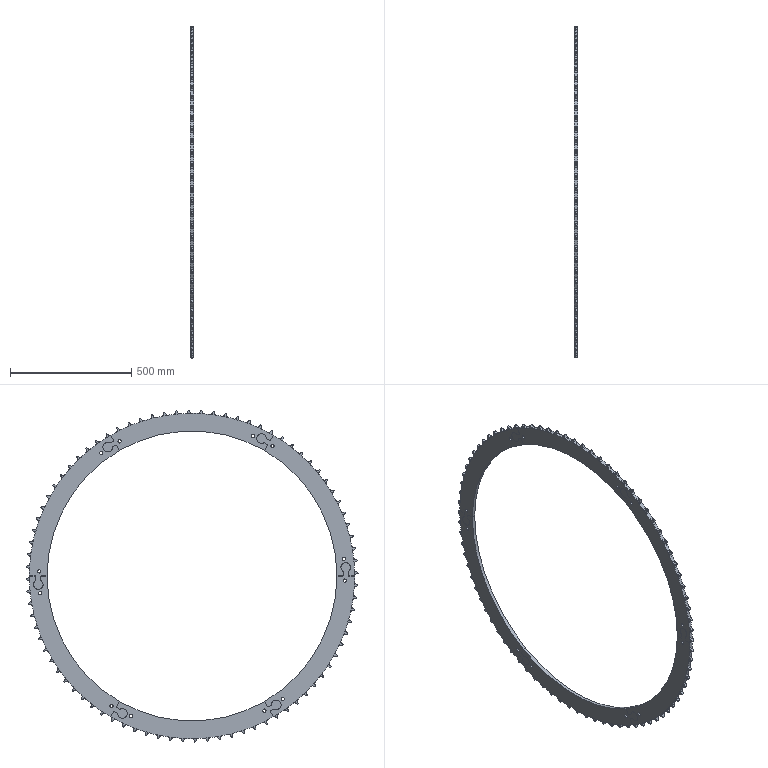Part | SolidWorks | features CirPattern 2, ICE 2, Cut 1, HoleWzd 1, Revolution 1 | 6 solids | 1212 faces | box 14.048 x 1371 x 1371 mm | volume 4173248 mm3 | cylinder 816 | plane 228 | torus 168 | commonest cylinder face diameters 22.306 x192 16.059 x174 41.467 x168 1343 x84 1371 x84 4 x54